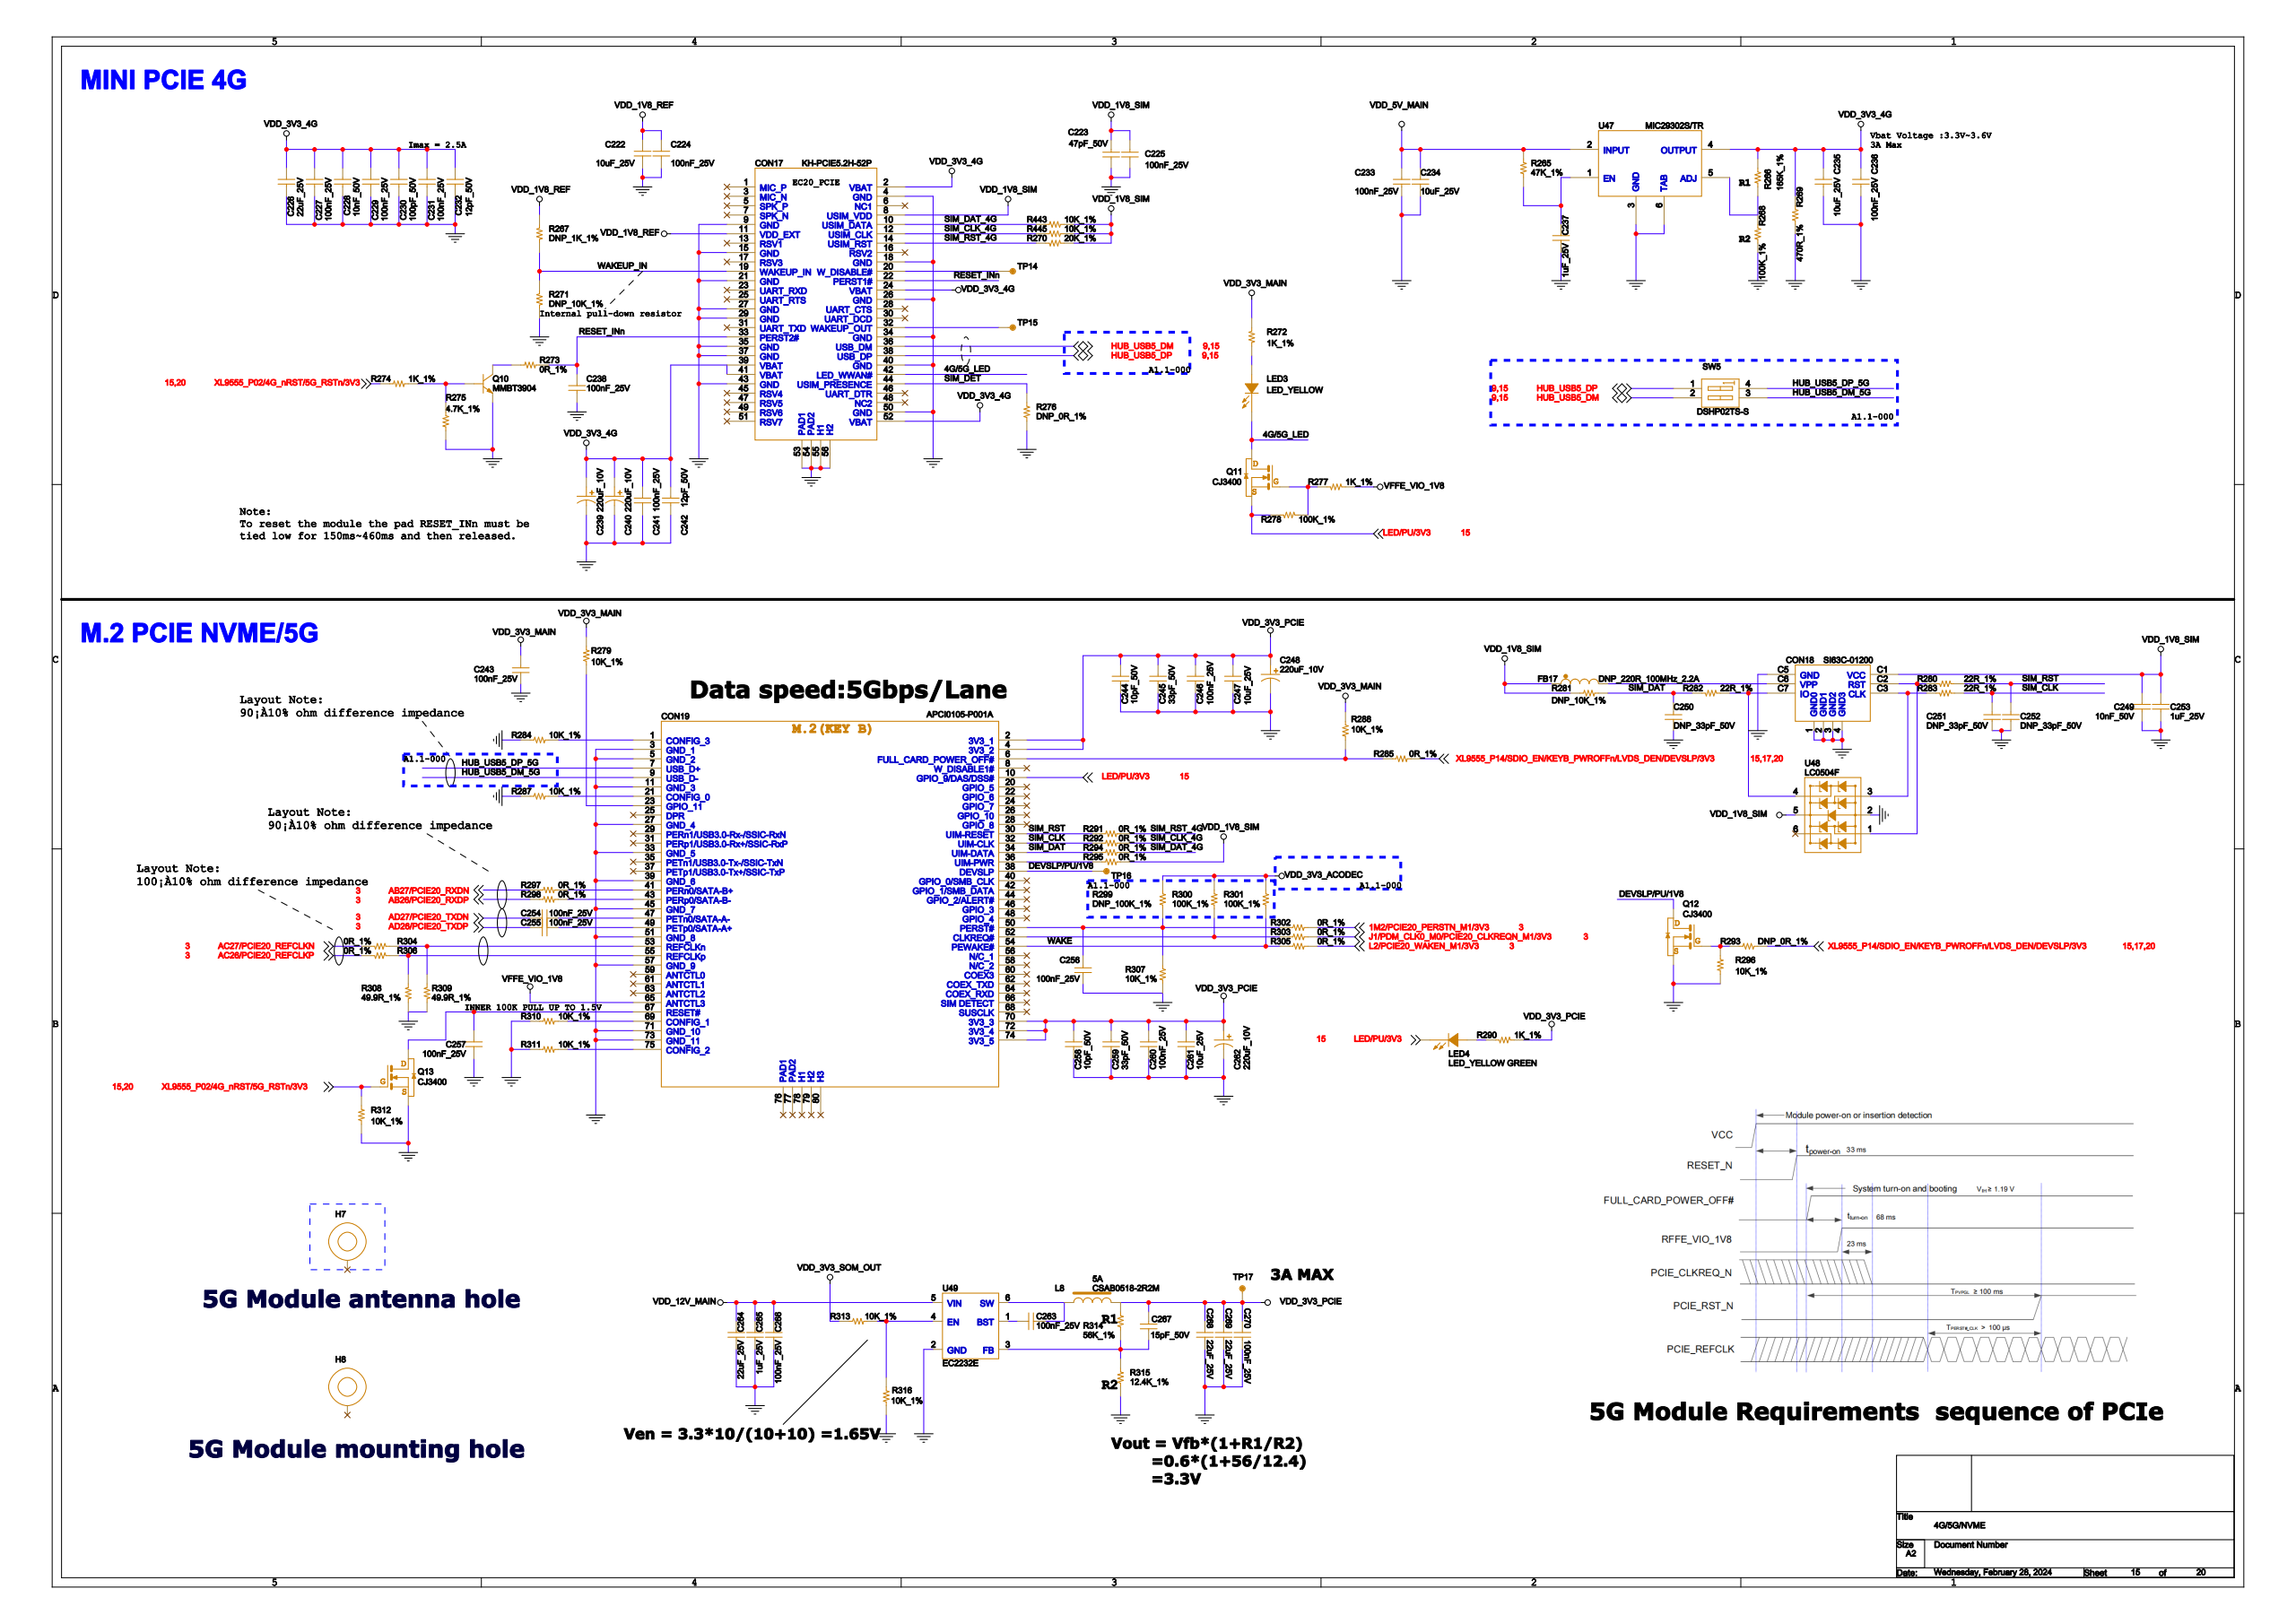Circuit board | Cadence Allegro | 1024 parts | 682 nets | one sheet of the schematic
Parts on this sheet (reference | value | footprint):
C222 | 10uF_25V | C0603
C223 | 47pF_50V | C0603
C224 | 100nF_25V | C0402
C225 | 100nF_25V | C0402
C226 | 22uF_25V | C0805
C227 | 100nF_25V | C0402
C228 | 10nF_50V | C0402
C229 | 100nF_25V | C0402
C230 | 100pF_50V | C0603
C231 | 100nF_25V | C0402
C232 | 12pF_50V | C0402
C233 | 100nF_25V | C0402
C234 | 10uF_25V | C0603
C235 | 10uF_25V | C0603
C236 | 100nF_25V | C0402
C237 | 1uF_25V | C0603
C238 | 100nF_25V | C0402
C239 | 220uF_10V | CAP_CASE_D
C240 | 220uF_10V | CAP_CASE_D
C241 | 100nF_25V | C0402
C242 | 12pF_50V | C0402
C243 | 100nF_25V | C0402
C244 | 10pF_25V | C0603
C245 | 33pF_50V | C0603
C246 | 100nF_25V | C0402
C247 | 10uF_25V | C0603
C248 | 220uF_10V | CAP_CASE_D
C249 | 10nF_50V | C0402
C250 | DNP_33pF_50V | C0603
C251 | DNP_33pF_50V | C0603
C252 | DNP_33pF_50V | C0603
C253 | 1uF_25V | C0603
C254 | 100nF_25V | C0402
C255 | 100nF_25V | C0402
C256 | 100nF_25V | C0402
C257 | 100nF_25V | C0402
C258 | 10pF_25V | C0603
C259 | 33pF_50V | C0603
C260 | 100nF_25V | C0402
C261 | 10uF_25V | C0603
C262 | 220uF_10V | CAP_CASE_D
C263 | 100nF_25V | C0402
C264 | 22uF_25V | C0805
C265 | 1uF_25V | C0603
C266 | 100nF_25V | C0402
C267 | 15pF_50V | C0402
C268 | 22uF_25V | C0805
C269 | 22uF_25V | C0805
C270 | 100nF_25V | C0402
CON17 | KH-PCIE5.2H-52P | CON_MINI_PCIE_4G
CON18 | SI63C-01200 | MICRO-SIM
CON19 | CON_M_2 | CONN-SMD_APCI0103-P001A
FB17 | DNP_220R_100MHz_2A | L0603
L8 | CSAB0518-2R2M | SMD_CSAB0518
LED3 | YELLOW_LED | CON_2P_3MM
LED4 | LED_GREEN | D0603
Q10 | MMBT3904 | SOT23-3_DBZ3
Q11 | CJ3400 | SOT23-3_DBZ3
Q12 | CJ3400 | SOT23-3_DBZ3
Q13 | CJ3400 | SOT23-3_DBZ3
R265 | 47K_1% | R0402
R266 | 165K_1% | R0603
R267 | DNP_1K_1% | R0402
R268 | 100K_1% | R0402
R269 | 470R_1% | R0805
R270 | 20K_1% | R0402
R271 | DNP_10K_1% | R0402
R272 | 1K_1% | R0402
R273 | 0R_1% | R0402
R274 | 1K_1% | R0402
R275 | 4.7K_1% | R0402
R276 | DNP_0R_1% | R0402
R277 | 1K_1% | R0402
R278 | 100K_1% | R0402
R279 | 10K_1% | R0402
R280 | 22R_1% | R0402
R281 | DNP_10K_1% | R0402
R282 | 22R_1% | R0402
R283 | 22R_1% | R0402
R284 | 10K_1% | R0402
R285 | 0R_1% | R0402
R287 | 10K_1% | R0402
R288 | 10K_1% | R0402
R290 | 1K_1% | R0402
R291 | 0R_1% | R0402
R292 | 0R_1% | R0402
R293 | DNP_0R_1% | R0402
R294 | 0R_1% | R0402
R295 | 0R_1% | R0603
R296 | 10K_1% | R0402
R297 | 0R_1% | R0402
R298 | 0R_1% | R0402
R299 | DNP_100K_1% | R0402
R300 | 100K_1% | R0402
R301 | 100K_1% | R0402
R302 | 0R_1% | R0402
R303 | 0R_1% | R0402
R304 | 0R_1% | R0402
R305 | 0R_1% | R0402
R306 | 0R_1% | R0402
R307 | 10K_1% | R0402
R308 | 49.9R_1% | R0603
R309 | 49.9R_1% | R0603
R310 | 10K_1% | R0402
R311 | 10K_1% | R0402
R312 | 10K_1% | R0402
R313 | 10K_1% | R0402
R314 | 56K_1% | R0402
R315 | 12.4K_1% | R0402
R316 | 10K_1% | R0402
R443 | 10K_1% | R0402
R445 | 10K_1% | R0402
SW5 | DSHP02TS-S Switch | DSHP02TS
TP14 | SMT TP | TP30
TP15 | SMT TP | TP30
TP16 | SMT TP | TP30
TP17 | SMT TP | TP30
U47 | MIC29302S/TR | TO-263
U48 | LC0504F | SOT363
U49 | EC2232E | SOT-23-6L
Nets of these parts (net: part-pin ...):
HUB_USB5_DP: SW5-1 CON17-38
HUB_USB5_DM: SW5-2 CON17-36
HUB_USB5_DP_5G: SW5-4 CON19-7
HUB_USB5_DM_5G: SW5-3 CON19-9
GND: C222-2 C223-1 C224-2 C225-1 C226-2 C227-2 C228-2 C229-2 C230-2 C231-2 C232-2 C233-2 C234-2 C235-2 C236-2 C237-2 C238-2 C239-2 C240-2 C241-2 C242-2 C243-1 C244-2 C245-2 C246-2 C247-2 C248-2 C249-2 C250-1 C251-1 C252-1 C253-2 C256-1 C257-2 C258-2 C259-2 C260-2 C261-2 C262-2 C264-2 C265-2 C266-2 C268-2 C269-2 C270-2 CON18-1 CON18-2 CON18-3 CON18-4 CON18-C5 Q10-2 Q12-2 Q13-2 R268-1 R269-1 R271-2 R275-1 R276-2 R284-2 R287-2 R296-2 R307-2 R308-1 R309-1 R310-2 R311-2 R312-2 R315-1 R316-1 U47-3 U47-6 U48-2 U49-2 CON17-4 CON17-9 CON17-15 CON17-18 CON17-21 CON17-26 CON17-27 CON17-29 CON17-34 CON17-35 CON17-37 CON17-40 CON17-43 CON17-50 CON17-53 CON17-54 CON17-55 CON17-56 CON19-3 CON19-5 CON19-11 CON19-27 CON19-33 CON19-39 CON19-45 CON19-51 CON19-57 CON19-71 CON19-73
VDD_5V_MAIN: C233-1 C234-1 R265-2 U47-2
VDD_3V3_ACODEC: R299-1 R300-1 R301-1
N21686255: C256-2 R299-2 R302-2 R307-1 CON19-50
VDD_3V3_MAIN: C243-2 R272-2 R279-1 R288-1
N21808885: C267-1 R314-1 R315-2 U49-3
VDD_3V3_PCIE: C244-1 C245-1 C246-1 C247-1 C248-1 C258-1 C259-1 C260-1 C261-1 C262-1 C267-2 C268-1 C269-1 C270-1 L8-2 R290-1 R314-2 TP17-1 CON19-2 CON19-4 CON19-70 CON19-72 CON19-74
VDD_3V3_4G: C226-1 C227-1 C228-1 C229-1 C230-1 C231-1 C232-1 C235-1 C236-1 C239-1 C240-1 C241-1 C242-1 R266-1 R269-2 U47-4 CON17-2 CON17-24 CON17-39 CON17-41 CON17-52
VDD_1V8_SIM: C223-2 C225-2 C249-1 C253-1 CON18-C1 FB17-1 R270-2 R281-1 R295-1 R443-2 R445-2 U48-5 CON17-8
AD26/PCIE20_TXDP: C255-2
AD27/PCIE20_TXDN: C254-2
AB26/PCIE20_RXDP: R298-1
AB27/PCIE20_RXDN: R297-1
VDD_3V3_SOM_OUT: R313-2
L2/PCIE20_WAKEN_M1/3V3: R305-1
1M2/PCIE20_PERSTN_M1/3V3: R302-1
J1/PDM_CLK0_M0/PCIE20_CLKREQN_M: R303-1
4G/5G_LED: LED3-2 Q11-3 CON17-42
RESET_INN: C238-1 R273-2 CON17-22 CON17-33
SIM_CLK_4G: R292-1 R445-1 CON17-12
SIM_DAT_4G: R294-1 R443-1 CON17-10
SIM_DET: R276-1 CON17-44
SIM_RST_4G: R270-1 R291-1 CON17-14
VDD_1V8_REF: C222-1 C224-1 R267-1 CON17-11
WAKEUP_IN: R267-2 R271-1 CON17-19
N21615690: TP15-1 CON17-32
N21615743: TP14-1 CON17-20
VFFE_VIO_1V8: R277-1 CON19-65
N21686528: R300-2 R303-2 CON19-52
N21686476: R287-1 CON19-21
N21686488: R310-1 CON19-69
N21686486: R311-1 CON19-75
N21686682: R284-1 CON19-1
DEVSLP/PU/1V8: Q12-3 TP16-1 CON19-38
N21686519: R285-2 R288-2 CON19-6
N21686521: R279-2 CON19-23
LED/PU/3V3: LED4-2 Q11-2 R278-2 CON19-10
N21686624: R297-2 CON19-41
N21686622: R298-2 CON19-43
N21686358: C254-1 CON19-47
N21686356: C255-1 CON19-49
WAKE: R301-2 R305-2 CON19-54
N21686403: R304-1 R309-2 CON19-53
N21686423: R306-1 R308-2 CON19-55
N21686282: C257-1 Q13-3 CON19-67
SIM_CLK: C251-2 R283-2 R292-2 CON19-32
SIM_DAT: C250-2 R281-2 R282-1 R294-2 CON19-34
N21908144: R295-2 CON19-36
SIM_RST: C252-2 R280-2 R291-2 CON19-30
VDD_12V_MAIN: C264-1 C265-1 C266-1 U49-5
N21629899: R266-2 R268-2 U47-5
N21906809: Q11-1 R277-2 R278-1
N21629915: C237-1 R265-1 U47-1
N21616485: Q10-3 R273-1
N21906775: LED3-1 R272-1
N21616471: Q10-1 R274-1 R275-2
XL9555_P02/4G_NRST/5G_RSTN/3V3: Q13-1 R274-2 R312-1
N21907536: LED4-1 R290-2
XL9555_P14/SDIO_EN/KEYB_PWROFFN: R285-1 R293-2
N21686765: CON18-C2 R280-1 U48-1
N21686253: CON18-C7 R282-2 U48-4
N21686700: CON18-C3 R283-1 U48-3
AC26/PCIE20_REFCLKP: R306-2
AC27/PCIE20_REFCLKN: R304-2
N21686185: Q12-1 R293-1 R296-1
N21808871: C263-2 L8-1 U49-6
N21808881: C263-1 U49-1
N21686728: CON18-C6 FB17-2
N21808785: R313-1 R316-2 U49-4